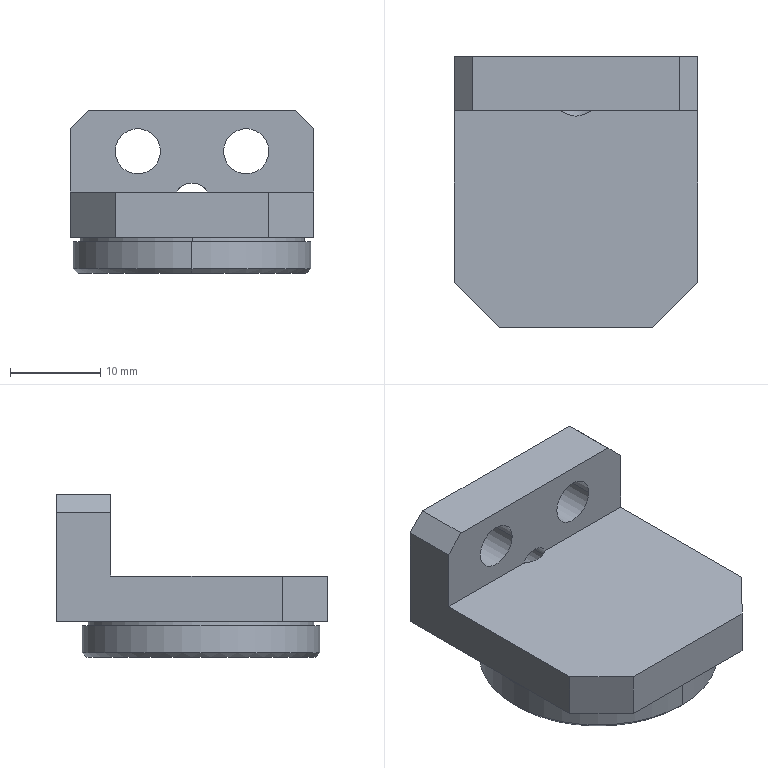NC program | NX | posted with a generic post | part box 27 x 30 x 18 mm
Whole program, first 1632 of 1946 lines:
N10 G17 G21 G94 G90
(FLOOR_WALL , TOOL : D10JING)
N12 T11 M6
N14 G54
N16 G17 G0 G90 X27. Y-17.497 B0. C0. S9500 M3
N18 G43 Z30. H11
N20 Z3.
N22 G94 G1 Z0. F1250.
N24 X24.
N26 X-24.
N28 Y-13.069
N30 X24.
N32 Y-8.641
N34 X-24.
N36 Y-4.213
N38 X24.
N40 Y0.216
N42 X-24.
N44 Y4.644
N46 X24.
N48 Y9.072
N50 X-24.
N52 Y13.5
N54 X24.
N56 X27.
N58 Z3.
N60 G0 Z30.
N62 M5
(ZLEVEL_PROFILE , TOOL : D10)
N64 T10 M6
N66 G54
N68 G17 G0 G90 X17.147 Y13.566 B0. C0. S9500 M3
N70 G43 Z30. H10
N72 Z1.5
N74 G94 G1 X18.832 Y11.88 Z1.375 F1000.
N76 X19.336 Y11.205 Z1.331
N78 X19.721 Y10.456 Z1.287
N80 X19.978 Y9.653 Z1.243
N82 X20.1 Y8.82 Z1.198
N84 Y-8.82 Z0.274
N86 X19.978 Y-9.653 Z0.23
N88 X19.721 Y-10.456 Z0.186
N90 X19.336 Y-11.205 Z0.142
N92 X18.832 Y-11.88 Z0.097
N94 X13.38 Y-17.332 Z-0.307
N96 X12.705 Y-17.836 Z-0.351
N98 X11.956 Y-18.221 Z-0.395
N100 X11.153 Y-18.478 Z-0.439
N102 X10.32 Y-18.6 Z-0.483
N104 X10. Z-0.5
N106 X-15. F3000.
N108 G2 X-20.1 Y-13.5 R5.1
N110 G1 Y13.5
N112 G2 X-15. Y18.6 R5.1
N114 G1 X10.
N116 G2 X13.606 Y17.106 R5.1
N118 G1 X18.606 Y12.106
N120 G2 X20.1 Y8.5 R5.1
N122 G1 Y-8.5
N124 G2 X18.606 Y-12.106 R5.1
N126 G1 X13.606 Y-17.106
N128 G2 X10. Y-18.6 R5.1
N130 G1 X-14.679 Z-0.931
N132 X-14.899 Z-0.935
N134 X-15.119 Y-18.599 Z-0.938
N136 X-15.34 Y-18.589 Z-0.942
N138 X-15.559 Y-18.569 Z-0.946
N140 X-15.777 Y-18.54 Z-0.95
N142 X-15.994 Y-18.502 Z-0.954
N144 X-16.21 Y-18.454 Z-0.958
N146 X-16.422 Y-18.398 Z-0.962
N148 X-16.633 Y-18.332 Z-0.965
N150 X-16.84 Y-18.257 Z-0.969
N152 X-17.044 Y-18.173 Z-0.973
N154 X-17.243 Y-18.08 Z-0.977
N156 X-17.439 Y-17.979 Z-0.981
N158 X-17.63 Y-17.869 Z-0.985
N160 X-17.817 Y-17.752 Z-0.988
N162 X-17.998 Y-17.626 Z-0.992
N164 X-18.173 Y-17.493 Z-0.996
N166 X-18.343 Y-17.352 Z-1.
N168 G2 X-20.1 Y-13.5 R5.1
N170 G1 Y13.5
N172 G2 X-15. Y18.6 R5.1
N174 G1 X10.
N176 G2 X13.606 Y17.106 R5.1
N178 G1 X18.606 Y12.106
N180 G2 X20.1 Y8.5 R5.1
N182 G1 Y-8.5
N184 G2 X18.606 Y-12.106 R5.1
N186 G1 X13.606 Y-17.106
N188 G2 X10. Y-18.6 R5.1
N190 G1 X-14.679 Z-1.431
N192 X-14.899 Z-1.435
N194 X-15.119 Y-18.599 Z-1.438
N196 X-15.34 Y-18.589 Z-1.442
N198 X-15.559 Y-18.569 Z-1.446
N200 X-15.777 Y-18.54 Z-1.45
N202 X-15.994 Y-18.502 Z-1.454
N204 X-16.21 Y-18.454 Z-1.458
N206 X-16.422 Y-18.398 Z-1.462
N208 X-16.633 Y-18.332 Z-1.465
N210 X-16.84 Y-18.257 Z-1.469
N212 X-17.044 Y-18.173 Z-1.473
N214 X-17.243 Y-18.08 Z-1.477
N216 X-17.439 Y-17.979 Z-1.481
N218 X-17.63 Y-17.869 Z-1.485
N220 X-17.817 Y-17.752 Z-1.488
N222 X-17.998 Y-17.626 Z-1.492
N224 X-18.173 Y-17.493 Z-1.496
N226 X-18.343 Y-17.352 Z-1.5
N228 G2 X-20.1 Y-13.5 R5.1
N230 G1 Y13.5
N232 G2 X-15. Y18.6 R5.1
N234 G1 X10.
N236 G2 X13.606 Y17.106 R5.1
N238 G1 X18.606 Y12.106
N240 G2 X20.1 Y8.5 R5.1
N242 G1 Y-8.5
N244 G2 X18.606 Y-12.106 R5.1
N246 G1 X13.606 Y-17.106
N248 G2 X10. Y-18.6 R5.1
N250 G1 X-14.679 Z-1.931
N252 X-14.899 Z-1.935
N254 X-15.119 Y-18.599 Z-1.938
N256 X-15.34 Y-18.589 Z-1.942
N258 X-15.559 Y-18.569 Z-1.946
N260 X-15.777 Y-18.54 Z-1.95
N262 X-15.994 Y-18.502 Z-1.954
N264 X-16.21 Y-18.454 Z-1.958
N266 X-16.422 Y-18.398 Z-1.962
N268 X-16.633 Y-18.332 Z-1.965
N270 X-16.84 Y-18.257 Z-1.969
N272 X-17.044 Y-18.173 Z-1.973
N274 X-17.243 Y-18.08 Z-1.977
N276 X-17.439 Y-17.979 Z-1.981
N278 X-17.63 Y-17.869 Z-1.985
N280 X-17.817 Y-17.752 Z-1.988
N282 X-17.998 Y-17.626 Z-1.992
N284 X-18.173 Y-17.493 Z-1.996
N286 X-18.343 Y-17.352 Z-2.
N288 G2 X-20.1 Y-13.5 R5.1
N290 G1 Y13.5
N292 G2 X-15. Y18.6 R5.1
N294 G1 X10.
N296 G2 X13.606 Y17.106 R5.1
N298 G1 X18.606 Y12.106
N300 G2 X20.1 Y8.5 R5.1
N302 G1 Y-8.5
N304 G2 X18.606 Y-12.106 R5.1
N306 G1 X13.606 Y-17.106
N308 G2 X10. Y-18.6 R5.1
N310 G1 X-14.679 Z-2.431
N312 X-14.899 Z-2.435
N314 X-15.119 Y-18.599 Z-2.438
N316 X-15.34 Y-18.589 Z-2.442
N318 X-15.559 Y-18.569 Z-2.446
N320 X-15.777 Y-18.54 Z-2.45
N322 X-15.994 Y-18.502 Z-2.454
N324 X-16.21 Y-18.454 Z-2.458
N326 X-16.422 Y-18.398 Z-2.462
N328 X-16.633 Y-18.332 Z-2.465
N330 X-16.84 Y-18.257 Z-2.469
N332 X-17.044 Y-18.173 Z-2.473
N334 X-17.243 Y-18.08 Z-2.477
N336 X-17.439 Y-17.979 Z-2.481
N338 X-17.63 Y-17.869 Z-2.485
N340 X-17.817 Y-17.752 Z-2.488
N342 X-17.998 Y-17.626 Z-2.492
N344 X-18.173 Y-17.493 Z-2.496
N346 X-18.343 Y-17.352 Z-2.5
N348 G2 X-20.1 Y-13.5 R5.1
N350 G1 Y13.5
N352 G2 X-15. Y18.6 R5.1
N354 G1 X10.
N356 G2 X13.606 Y17.106 R5.1
N358 G1 X18.606 Y12.106
N360 G2 X20.1 Y8.5 R5.1
N362 G1 Y-8.5
N364 G2 X18.606 Y-12.106 R5.1
N366 G1 X13.606 Y-17.106
N368 G2 X10. Y-18.6 R5.1
N370 G1 X-14.679 Z-2.931
N372 X-14.899 Z-2.935
N374 X-15.119 Y-18.599 Z-2.938
N376 X-15.34 Y-18.589 Z-2.942
N378 X-15.559 Y-18.569 Z-2.946
N380 X-15.777 Y-18.54 Z-2.95
N382 X-15.994 Y-18.502 Z-2.954
N384 X-16.21 Y-18.454 Z-2.958
N386 X-16.422 Y-18.398 Z-2.962
N388 X-16.633 Y-18.332 Z-2.965
N390 X-16.84 Y-18.257 Z-2.969
N392 X-17.044 Y-18.173 Z-2.973
N394 X-17.243 Y-18.08 Z-2.977
N396 X-17.439 Y-17.979 Z-2.981
N398 X-17.63 Y-17.869 Z-2.985
N400 X-17.817 Y-17.752 Z-2.988
N402 X-17.998 Y-17.626 Z-2.992
N404 X-18.173 Y-17.493 Z-2.996
N406 X-18.343 Y-17.352 Z-3.
N408 G2 X-20.1 Y-13.5 R5.1
N410 G1 Y13.5
N412 G2 X-15. Y18.6 R5.1
N414 G1 X10.
N416 G2 X13.606 Y17.106 R5.1
N418 G1 X18.606 Y12.106
N420 G2 X20.1 Y8.5 R5.1
N422 G1 Y-8.5
N424 G2 X18.606 Y-12.106 R5.1
N426 G1 X13.606 Y-17.106
N428 G2 X10. Y-18.6 R5.1
N430 G1 X-14.679 Z-3.431
N432 X-14.899 Z-3.435
N434 X-15.119 Y-18.599 Z-3.438
N436 X-15.34 Y-18.589 Z-3.442
N438 X-15.559 Y-18.569 Z-3.446
N440 X-15.777 Y-18.54 Z-3.45
N442 X-15.994 Y-18.502 Z-3.454
N444 X-16.21 Y-18.454 Z-3.458
N446 X-16.422 Y-18.398 Z-3.462
N448 X-16.633 Y-18.332 Z-3.465
N450 X-16.84 Y-18.257 Z-3.469
N452 X-17.044 Y-18.173 Z-3.473
N454 X-17.243 Y-18.08 Z-3.477
N456 X-17.439 Y-17.979 Z-3.481
N458 X-17.63 Y-17.869 Z-3.485
N460 X-17.817 Y-17.752 Z-3.488
N462 X-17.998 Y-17.626 Z-3.492
N464 X-18.173 Y-17.493 Z-3.496
N466 X-18.343 Y-17.352 Z-3.5
N468 G2 X-20.1 Y-13.5 R5.1
N470 G1 Y13.5
N472 G2 X-15. Y18.6 R5.1
N474 G1 X10.
N476 G2 X13.606 Y17.106 R5.1
N478 G1 X18.606 Y12.106
N480 G2 X20.1 Y8.5 R5.1
N482 G1 Y-8.5
N484 G2 X18.606 Y-12.106 R5.1
N486 G1 X13.606 Y-17.106
N488 G2 X10. Y-18.6 R5.1
N490 G1 X-14.679 Z-3.931
N492 X-14.899 Z-3.935
N494 X-15.119 Y-18.599 Z-3.938
N496 X-15.34 Y-18.589 Z-3.942
N498 X-15.559 Y-18.569 Z-3.946
N500 X-15.777 Y-18.54 Z-3.95
N502 X-15.994 Y-18.502 Z-3.954
N504 X-16.21 Y-18.454 Z-3.958
N506 X-16.422 Y-18.398 Z-3.962
N508 X-16.633 Y-18.332 Z-3.965
N510 X-16.84 Y-18.257 Z-3.969
N512 X-17.044 Y-18.173 Z-3.973
N514 X-17.243 Y-18.08 Z-3.977
N516 X-17.439 Y-17.979 Z-3.981
N518 X-17.63 Y-17.869 Z-3.985
N520 X-17.817 Y-17.752 Z-3.988
N522 X-17.998 Y-17.626 Z-3.992
N524 X-18.173 Y-17.493 Z-3.996
N526 X-18.343 Y-17.352 Z-4.
N528 G2 X-20.1 Y-13.5 R5.1
N530 G1 Y13.5
N532 G2 X-15. Y18.6 R5.1
N534 G1 X10.
N536 G2 X13.606 Y17.106 R5.1
N538 G1 X18.606 Y12.106
N540 G2 X20.1 Y8.5 R5.1
N542 G1 Y-8.5
N544 G2 X18.606 Y-12.106 R5.1
N546 G1 X13.606 Y-17.106
N548 G2 X10. Y-18.6 R5.1
N550 G1 X-14.679 Z-4.431
N552 X-14.899 Z-4.435
N554 X-15.119 Y-18.599 Z-4.438
N556 X-15.34 Y-18.589 Z-4.442
N558 X-15.559 Y-18.569 Z-4.446
N560 X-15.777 Y-18.54 Z-4.45
N562 X-15.994 Y-18.502 Z-4.454
N564 X-16.21 Y-18.454 Z-4.458
N566 X-16.422 Y-18.398 Z-4.462
N568 X-16.633 Y-18.332 Z-4.465
N570 X-16.84 Y-18.257 Z-4.469
N572 X-17.044 Y-18.173 Z-4.473
N574 X-17.243 Y-18.08 Z-4.477
N576 X-17.439 Y-17.979 Z-4.481
N578 X-17.63 Y-17.869 Z-4.485
N580 X-17.817 Y-17.752 Z-4.488
N582 X-17.998 Y-17.626 Z-4.492
N584 X-18.173 Y-17.493 Z-4.496
N586 X-18.343 Y-17.352 Z-4.5
N588 G2 X-20.1 Y-13.5 R5.1
N590 G1 Y13.5
N592 G2 X-15. Y18.6 R5.1
N594 G1 X10.
N596 G2 X13.606 Y17.106 R5.1
N598 G1 X18.606 Y12.106
N600 G2 X20.1 Y8.5 R5.1
N602 G1 Y-8.5
N604 G2 X18.606 Y-12.106 R5.1
N606 G1 X13.606 Y-17.106
N608 G2 X10. Y-18.6 R5.1
N610 G1 X-14.679 Z-4.931
N612 X-14.899 Z-4.935
N614 X-15.119 Y-18.599 Z-4.938
N616 X-15.34 Y-18.589 Z-4.942
N618 X-15.559 Y-18.569 Z-4.946
N620 X-15.777 Y-18.54 Z-4.95
N622 X-15.994 Y-18.502 Z-4.954
N624 X-16.21 Y-18.454 Z-4.958
N626 X-16.422 Y-18.398 Z-4.962
N628 X-16.633 Y-18.332 Z-4.965
N630 X-16.84 Y-18.257 Z-4.969
N632 X-17.044 Y-18.173 Z-4.973
N634 X-17.243 Y-18.08 Z-4.977
N636 X-17.439 Y-17.979 Z-4.981
N638 X-17.63 Y-17.869 Z-4.985
N640 X-17.817 Y-17.752 Z-4.988
N642 X-17.998 Y-17.626 Z-4.992
N644 X-18.173 Y-17.493 Z-4.996
N646 X-18.343 Y-17.352 Z-5.
N648 G2 X-20.1 Y-13.5 R5.1
N650 G1 Y13.5
N652 G2 X-15. Y18.6 R5.1
N654 G1 X10.
N656 G2 X13.606 Y17.106 R5.1
N658 G1 X18.606 Y12.106
N660 G2 X20.1 Y8.5 R5.1
N662 G1 Y-8.5
N664 G2 X18.606 Y-12.106 R5.1
N666 G1 X13.606 Y-17.106
N668 G2 X10. Y-18.6 R5.1
N670 G1 X-14.679 Z-5.431
N672 X-14.899 Z-5.435
N674 X-15.119 Y-18.599 Z-5.438
N676 X-15.34 Y-18.589 Z-5.442
N678 X-15.559 Y-18.569 Z-5.446
N680 X-15.777 Y-18.54 Z-5.45
N682 X-15.994 Y-18.502 Z-5.454
N684 X-16.21 Y-18.454 Z-5.458
N686 X-16.422 Y-18.398 Z-5.462
N688 X-16.633 Y-18.332 Z-5.465
N690 X-16.84 Y-18.257 Z-5.469
N692 X-17.044 Y-18.173 Z-5.473
N694 X-17.243 Y-18.08 Z-5.477
N696 X-17.439 Y-17.979 Z-5.481
N698 X-17.63 Y-17.869 Z-5.485
N700 X-17.817 Y-17.752 Z-5.488
N702 X-17.998 Y-17.626 Z-5.492
N704 X-18.173 Y-17.493 Z-5.496
N706 X-18.343 Y-17.352 Z-5.5
N708 G2 X-20.1 Y-13.5 R5.1
N710 G1 Y13.5
N712 G2 X-15. Y18.6 R5.1
N714 G1 X10.
N716 G2 X13.606 Y17.106 R5.1
N718 G1 X18.606 Y12.106
N720 G2 X20.1 Y8.5 R5.1
N722 G1 Y-8.5
N724 G2 X18.606 Y-12.106 R5.1
N726 G1 X13.606 Y-17.106
N728 G2 X10. Y-18.6 R5.1
N730 G1 X-14.679 Z-5.931
N732 X-14.899 Z-5.935
N734 X-15.119 Y-18.599 Z-5.938
N736 X-15.34 Y-18.589 Z-5.942
N738 X-15.559 Y-18.569 Z-5.946
N740 X-15.777 Y-18.54 Z-5.95
N742 X-15.994 Y-18.502 Z-5.954
N744 X-16.21 Y-18.454 Z-5.958
N746 X-16.422 Y-18.398 Z-5.962
N748 X-16.633 Y-18.332 Z-5.965
N750 X-16.84 Y-18.257 Z-5.969
N752 X-17.044 Y-18.173 Z-5.973
N754 X-17.243 Y-18.08 Z-5.977
N756 X-17.439 Y-17.979 Z-5.981
N758 X-17.63 Y-17.869 Z-5.985
N760 X-17.817 Y-17.752 Z-5.988
N762 X-17.998 Y-17.626 Z-5.992
N764 X-18.173 Y-17.493 Z-5.996
N766 X-18.343 Y-17.352 Z-6.
N768 G2 X-20.1 Y-13.5 R5.1
N770 G1 Y13.5
N772 G2 X-15. Y18.6 R5.1
N774 G1 X10.
N776 G2 X13.606 Y17.106 R5.1
N778 G1 X18.606 Y12.106
N780 G2 X20.1 Y8.5 R5.1
N782 G1 Y-8.5
N784 G2 X18.606 Y-12.106 R5.1
N786 G1 X13.606 Y-17.106
N788 G2 X10. Y-18.6 R5.1
N790 G1 X-14.679 Z-6.431
N792 X-14.899 Z-6.435
N794 X-15.119 Y-18.599 Z-6.438
N796 X-15.34 Y-18.589 Z-6.442
N798 X-15.559 Y-18.569 Z-6.446
N800 X-15.777 Y-18.54 Z-6.45
N802 X-15.994 Y-18.502 Z-6.454
N804 X-16.21 Y-18.454 Z-6.458
N806 X-16.422 Y-18.398 Z-6.462
N808 X-16.633 Y-18.332 Z-6.465
N810 X-16.84 Y-18.257 Z-6.469
N812 X-17.044 Y-18.173 Z-6.473
N814 X-17.243 Y-18.08 Z-6.477
N816 X-17.439 Y-17.979 Z-6.481
N818 X-17.63 Y-17.869 Z-6.485
N820 X-17.817 Y-17.752 Z-6.488
N822 X-17.998 Y-17.626 Z-6.492
N824 X-18.173 Y-17.493 Z-6.496
N826 X-18.343 Y-17.352 Z-6.5
N828 G2 X-20.1 Y-13.5 R5.1
N830 G1 Y13.5
N832 G2 X-15. Y18.6 R5.1
N834 G1 X10.
N836 G2 X13.606 Y17.106 R5.1
N838 G1 X18.606 Y12.106
N840 G2 X20.1 Y8.5 R5.1
N842 G1 Y-8.5
N844 G2 X18.606 Y-12.106 R5.1
N846 G1 X13.606 Y-17.106
N848 G2 X10. Y-18.6 R5.1
N850 G1 X-14.679 Z-6.931
N852 X-14.899 Z-6.935
N854 X-15.119 Y-18.599 Z-6.938
N856 X-15.34 Y-18.589 Z-6.942
N858 X-15.559 Y-18.569 Z-6.946
N860 X-15.777 Y-18.54 Z-6.95
N862 X-15.994 Y-18.502 Z-6.954
N864 X-16.21 Y-18.454 Z-6.958
N866 X-16.422 Y-18.398 Z-6.962
N868 X-16.633 Y-18.332 Z-6.965
N870 X-16.84 Y-18.257 Z-6.969
N872 X-17.044 Y-18.173 Z-6.973
N874 X-17.243 Y-18.08 Z-6.977
N876 X-17.439 Y-17.979 Z-6.981
N878 X-17.63 Y-17.869 Z-6.985
N880 X-17.817 Y-17.752 Z-6.988
N882 X-17.998 Y-17.626 Z-6.992
N884 X-18.173 Y-17.493 Z-6.996
N886 X-18.343 Y-17.352 Z-7.
N888 G2 X-20.1 Y-13.5 R5.1
N890 G1 Y13.5
N892 G2 X-15. Y18.6 R5.1
N894 G1 X10.
N896 G2 X13.606 Y17.106 R5.1
N898 G1 X18.606 Y12.106
N900 G2 X20.1 Y8.5 R5.1
N902 G1 Y-8.5
N904 G2 X18.606 Y-12.106 R5.1
N906 G1 X13.606 Y-17.106
N908 G2 X10. Y-18.6 R5.1
N910 G1 X-14.679 Z-7.431
N912 X-14.899 Z-7.435
N914 X-15.119 Y-18.599 Z-7.438
N916 X-15.34 Y-18.589 Z-7.442
N918 X-15.559 Y-18.569 Z-7.446
N920 X-15.777 Y-18.54 Z-7.45
N922 X-15.994 Y-18.502 Z-7.454
N924 X-16.21 Y-18.454 Z-7.458
N926 X-16.422 Y-18.398 Z-7.462
N928 X-16.633 Y-18.332 Z-7.465
N930 X-16.84 Y-18.257 Z-7.469
N932 X-17.044 Y-18.173 Z-7.473
N934 X-17.243 Y-18.08 Z-7.477
N936 X-17.439 Y-17.979 Z-7.481
N938 X-17.63 Y-17.869 Z-7.485
N940 X-17.817 Y-17.752 Z-7.488
N942 X-17.998 Y-17.626 Z-7.492
N944 X-18.173 Y-17.493 Z-7.496
N946 X-18.343 Y-17.352 Z-7.5
N948 G2 X-20.1 Y-13.5 R5.1
N950 G1 Y13.5
N952 G2 X-15. Y18.6 R5.1
N954 G1 X10.
N956 G2 X13.606 Y17.106 R5.1
N958 G1 X18.606 Y12.106
N960 G2 X20.1 Y8.5 R5.1
N962 G1 Y-8.5
N964 G2 X18.606 Y-12.106 R5.1
N966 G1 X13.606 Y-17.106
N968 G2 X10. Y-18.6 R5.1
N970 G1 X-14.679 Z-7.931
N972 X-14.899 Z-7.935
N974 X-15.119 Y-18.599 Z-7.938
N976 X-15.34 Y-18.589 Z-7.942
N978 X-15.559 Y-18.569 Z-7.946
N980 X-15.777 Y-18.54 Z-7.95
N982 X-15.994 Y-18.502 Z-7.954
N984 X-16.21 Y-18.454 Z-7.958
N986 X-16.422 Y-18.398 Z-7.962
N988 X-16.633 Y-18.332 Z-7.965
N990 X-16.84 Y-18.257 Z-7.969
N992 X-17.044 Y-18.173 Z-7.973
N994 X-17.243 Y-18.08 Z-7.977
N996 X-17.439 Y-17.979 Z-7.981
N998 X-17.63 Y-17.869 Z-7.985
N1000 X-17.817 Y-17.752 Z-7.988
N1002 X-17.998 Y-17.626 Z-7.992
N1004 X-18.173 Y-17.493 Z-7.996
N1006 X-18.343 Y-17.352 Z-8.
N1008 G2 X-20.1 Y-13.5 R5.1
N1010 G1 Y13.5
N1012 G2 X-15. Y18.6 R5.1
N1014 G1 X10.
N1016 G2 X13.606 Y17.106 R5.1
N1018 G1 X18.606 Y12.106
N1020 G2 X20.1 Y8.5 R5.1
N1022 G1 Y-8.5
N1024 G2 X18.606 Y-12.106 R5.1
N1026 G1 X13.606 Y-17.106
N1028 G2 X10. Y-18.6 R5.1
N1030 G1 X-14.679 Z-8.431
N1032 X-14.899 Z-8.435
N1034 X-15.119 Y-18.599 Z-8.438
N1036 X-15.34 Y-18.589 Z-8.442
N1038 X-15.559 Y-18.569 Z-8.446
N1040 X-15.777 Y-18.54 Z-8.45
N1042 X-15.994 Y-18.502 Z-8.454
N1044 X-16.21 Y-18.454 Z-8.458
N1046 X-16.422 Y-18.398 Z-8.462
N1048 X-16.633 Y-18.332 Z-8.465
N1050 X-16.84 Y-18.257 Z-8.469
N1052 X-17.044 Y-18.173 Z-8.473
N1054 X-17.243 Y-18.08 Z-8.477
N1056 X-17.439 Y-17.979 Z-8.481
N1058 X-17.63 Y-17.869 Z-8.485
N1060 X-17.817 Y-17.752 Z-8.488
N1062 X-17.998 Y-17.626 Z-8.492
N1064 X-18.173 Y-17.493 Z-8.496
N1066 X-18.343 Y-17.352 Z-8.5
N1068 G2 X-20.1 Y-13.5 R5.1
N1070 G1 Y13.5
N1072 G2 X-15. Y18.6 R5.1
N1074 G1 X10.
N1076 G2 X13.606 Y17.106 R5.1
N1078 G1 X18.606 Y12.106
N1080 G2 X20.1 Y8.5 R5.1
N1082 G1 Y-8.5
N1084 G2 X18.606 Y-12.106 R5.1
N1086 G1 X13.606 Y-17.106
N1088 G2 X10. Y-18.6 R5.1
N1090 G1 X-14.679 Z-8.931
N1092 X-14.899 Z-8.935
N1094 X-15.119 Y-18.599 Z-8.938
N1096 X-15.34 Y-18.589 Z-8.942
N1098 X-15.559 Y-18.569 Z-8.946
N1100 X-15.777 Y-18.54 Z-8.95
N1102 X-15.994 Y-18.502 Z-8.954
N1104 X-16.21 Y-18.454 Z-8.958
N1106 X-16.422 Y-18.398 Z-8.962
N1108 X-16.633 Y-18.332 Z-8.965
N1110 X-16.84 Y-18.257 Z-8.969
N1112 X-17.044 Y-18.173 Z-8.973
N1114 X-17.243 Y-18.08 Z-8.977
N1116 X-17.439 Y-17.979 Z-8.981
N1118 X-17.63 Y-17.869 Z-8.985
N1120 X-17.817 Y-17.752 Z-8.988
N1122 X-17.998 Y-17.626 Z-8.992
N1124 X-18.173 Y-17.493 Z-8.996
N1126 X-18.343 Y-17.352 Z-9.
N1128 G2 X-20.1 Y-13.5 R5.1
N1130 G1 Y13.5
N1132 G2 X-15. Y18.6 R5.1
N1134 G1 X10.
N1136 G2 X13.606 Y17.106 R5.1
N1138 G1 X18.606 Y12.106
N1140 G2 X20.1 Y8.5 R5.1
N1142 G1 Y-8.5
N1144 G2 X18.606 Y-12.106 R5.1
N1146 G1 X13.606 Y-17.106
N1148 G2 X10. Y-18.6 R5.1
N1150 G1 X-14.679 Z-9.431
N1152 X-14.899 Z-9.435
N1154 X-15.119 Y-18.599 Z-9.438
N1156 X-15.34 Y-18.589 Z-9.442
N1158 X-15.559 Y-18.569 Z-9.446
N1160 X-15.777 Y-18.54 Z-9.45
N1162 X-15.994 Y-18.502 Z-9.454
N1164 X-16.21 Y-18.454 Z-9.458
N1166 X-16.422 Y-18.398 Z-9.462
N1168 X-16.633 Y-18.332 Z-9.465
N1170 X-16.84 Y-18.257 Z-9.469
N1172 X-17.044 Y-18.173 Z-9.473
N1174 X-17.243 Y-18.08 Z-9.477
N1176 X-17.439 Y-17.979 Z-9.481
N1178 X-17.63 Y-17.869 Z-9.485
N1180 X-17.817 Y-17.752 Z-9.488
N1182 X-17.998 Y-17.626 Z-9.492
N1184 X-18.173 Y-17.493 Z-9.496
N1186 X-18.343 Y-17.352 Z-9.5
N1188 G2 X-20.1 Y-13.5 R5.1
N1190 G1 Y13.5
N1192 G2 X-15. Y18.6 R5.1
N1194 G1 X10.
N1196 G2 X13.606 Y17.106 R5.1
N1198 G1 X18.606 Y12.106
N1200 G2 X20.1 Y8.5 R5.1
N1202 G1 Y-8.5
N1204 G2 X18.606 Y-12.106 R5.1
N1206 G1 X13.606 Y-17.106
N1208 G2 X10. Y-18.6 R5.1
N1210 G1 X-14.679 Z-9.931
N1212 X-14.899 Z-9.935
N1214 X-15.119 Y-18.599 Z-9.938
N1216 X-15.34 Y-18.589 Z-9.942
N1218 X-15.559 Y-18.569 Z-9.946
N1220 X-15.777 Y-18.54 Z-9.95
N1222 X-15.994 Y-18.502 Z-9.954
N1224 X-16.21 Y-18.454 Z-9.958
N1226 X-16.422 Y-18.398 Z-9.962
N1228 X-16.633 Y-18.332 Z-9.965
N1230 X-16.84 Y-18.257 Z-9.969
N1232 X-17.044 Y-18.173 Z-9.973
N1234 X-17.243 Y-18.08 Z-9.977
N1236 X-17.439 Y-17.979 Z-9.981
N1238 X-17.63 Y-17.869 Z-9.985
N1240 X-17.817 Y-17.752 Z-9.988
N1242 X-17.998 Y-17.626 Z-9.992
N1244 X-18.173 Y-17.493 Z-9.996
N1246 X-18.343 Y-17.352 Z-10.
N1248 G2 X-20.1 Y-13.5 R5.1
N1250 G1 Y13.5
N1252 G2 X-15. Y18.6 R5.1
N1254 G1 X10.
N1256 G2 X13.606 Y17.106 R5.1
N1258 G1 X18.606 Y12.106
N1260 G2 X20.1 Y8.5 R5.1
N1262 G1 Y-8.5
N1264 G2 X18.606 Y-12.106 R5.1
N1266 G1 X13.606 Y-17.106
N1268 G2 X10. Y-18.6 R5.1
N1270 G1 X-14.679 Z-10.431
N1272 X-14.899 Z-10.435
N1274 X-15.119 Y-18.599 Z-10.438
N1276 X-15.34 Y-18.589 Z-10.442
N1278 X-15.559 Y-18.569 Z-10.446
N1280 X-15.777 Y-18.54 Z-10.45
N1282 X-15.994 Y-18.502 Z-10.454
N1284 X-16.21 Y-18.454 Z-10.458
N1286 X-16.422 Y-18.398 Z-10.462
N1288 X-16.633 Y-18.332 Z-10.465
N1290 X-16.84 Y-18.257 Z-10.469
N1292 X-17.044 Y-18.173 Z-10.473
N1294 X-17.243 Y-18.08 Z-10.477
N1296 X-17.439 Y-17.979 Z-10.481
N1298 X-17.63 Y-17.869 Z-10.485
N1300 X-17.817 Y-17.752 Z-10.488
N1302 X-17.998 Y-17.626 Z-10.492
N1304 X-18.173 Y-17.493 Z-10.496
N1306 X-18.343 Y-17.352 Z-10.5
N1308 G2 X-20.1 Y-13.5 R5.1
N1310 G1 Y13.5
N1312 G2 X-15. Y18.6 R5.1
N1314 G1 X10.
N1316 G2 X13.606 Y17.106 R5.1
N1318 G1 X18.606 Y12.106
N1320 G2 X20.1 Y8.5 R5.1
N1322 G1 Y-8.5
N1324 G2 X18.606 Y-12.106 R5.1
N1326 G1 X13.606 Y-17.106
N1328 G2 X10. Y-18.6 R5.1
N1330 G1 X-14.679 Z-10.931
N1332 X-14.899 Z-10.935
N1334 X-15.119 Y-18.599 Z-10.938
N1336 X-15.34 Y-18.589 Z-10.942
N1338 X-15.559 Y-18.569 Z-10.946
N1340 X-15.777 Y-18.54 Z-10.95
N1342 X-15.994 Y-18.502 Z-10.954
N1344 X-16.21 Y-18.454 Z-10.958
N1346 X-16.422 Y-18.398 Z-10.962
N1348 X-16.633 Y-18.332 Z-10.965
N1350 X-16.84 Y-18.257 Z-10.969
N1352 X-17.044 Y-18.173 Z-10.973
N1354 X-17.243 Y-18.08 Z-10.977
N1356 X-17.439 Y-17.979 Z-10.981
N1358 X-17.63 Y-17.869 Z-10.985
N1360 X-17.817 Y-17.752 Z-10.988
N1362 X-17.998 Y-17.626 Z-10.992
N1364 X-18.173 Y-17.493 Z-10.996
N1366 X-18.343 Y-17.352 Z-11.
N1368 G2 X-20.1 Y-13.5 R5.1
N1370 G1 Y13.5
N1372 G2 X-15. Y18.6 R5.1
N1374 G1 X10.
N1376 G2 X13.606 Y17.106 R5.1
N1378 G1 X18.606 Y12.106
N1380 G2 X20.1 Y8.5 R5.1
N1382 G1 Y-8.5
N1384 G2 X18.606 Y-12.106 R5.1
N1386 G1 X13.606 Y-17.106
N1388 G2 X10. Y-18.6 R5.1
N1390 G1 X-14.679 Z-11.431
N1392 X-14.899 Z-11.435
N1394 X-15.119 Y-18.599 Z-11.438
N1396 X-15.34 Y-18.589 Z-11.442
N1398 X-15.559 Y-18.569 Z-11.446
N1400 X-15.777 Y-18.54 Z-11.45
N1402 X-15.994 Y-18.502 Z-11.454
N1404 X-16.21 Y-18.454 Z-11.458
N1406 X-16.422 Y-18.398 Z-11.462
N1408 X-16.633 Y-18.332 Z-11.465
N1410 X-16.84 Y-18.257 Z-11.469
N1412 X-17.044 Y-18.173 Z-11.473
N1414 X-17.243 Y-18.08 Z-11.477
N1416 X-17.439 Y-17.979 Z-11.481
N1418 X-17.63 Y-17.869 Z-11.485
N1420 X-17.817 Y-17.752 Z-11.488
N1422 X-17.998 Y-17.626 Z-11.492
N1424 X-18.173 Y-17.493 Z-11.496
N1426 X-18.343 Y-17.352 Z-11.5
N1428 G2 X-20.1 Y-13.5 R5.1
N1430 G1 Y13.5
N1432 G2 X-15. Y18.6 R5.1
N1434 G1 X10.
N1436 G2 X13.606 Y17.106 R5.1
N1438 G1 X18.606 Y12.106
N1440 G2 X20.1 Y8.5 R5.1
N1442 G1 Y-8.5
N1444 G2 X18.606 Y-12.106 R5.1
N1446 G1 X13.606 Y-17.106
N1448 G2 X10. Y-18.6 R5.1
N1450 G1 X-14.679 Z-11.931
N1452 X-14.899 Z-11.935
N1454 X-15.119 Y-18.599 Z-11.938
N1456 X-15.34 Y-18.589 Z-11.942
N1458 X-15.559 Y-18.569 Z-11.946
N1460 X-15.777 Y-18.54 Z-11.95
N1462 X-15.994 Y-18.502 Z-11.954
N1464 X-16.21 Y-18.454 Z-11.958
N1466 X-16.422 Y-18.398 Z-11.962
N1468 X-16.633 Y-18.332 Z-11.965
N1470 X-16.84 Y-18.257 Z-11.969
N1472 X-17.044 Y-18.173 Z-11.973
N1474 X-17.243 Y-18.08 Z-11.977
N1476 X-17.439 Y-17.979 Z-11.981
N1478 X-17.63 Y-17.869 Z-11.985
N1480 X-17.817 Y-17.752 Z-11.988
N1482 X-17.998 Y-17.626 Z-11.992
N1484 X-18.173 Y-17.493 Z-11.996
N1486 X-18.343 Y-17.352 Z-12.
N1488 G2 X-20.1 Y-13.5 R5.1
N1490 G1 Y13.5
N1492 G2 X-15. Y18.6 R5.1
N1494 G1 X10.
N1496 G2 X13.606 Y17.106 R5.1
N1498 G1 X18.606 Y12.106
N1500 G2 X20.1 Y8.5 R5.1
N1502 G1 Y-8.5
N1504 G2 X18.606 Y-12.106 R5.1
N1506 G1 X13.606 Y-17.106
N1508 G2 X10. Y-18.6 R5.1
N1510 G1 X-14.679 Z-12.431
N1512 X-14.899 Z-12.435
N1514 X-15.119 Y-18.599 Z-12.438
N1516 X-15.34 Y-18.589 Z-12.442
N1518 X-15.559 Y-18.569 Z-12.446
N1520 X-15.777 Y-18.54 Z-12.45
N1522 X-15.994 Y-18.502 Z-12.454
N1524 X-16.21 Y-18.454 Z-12.458
N1526 X-16.422 Y-18.398 Z-12.462
N1528 X-16.633 Y-18.332 Z-12.465
N1530 X-16.84 Y-18.257 Z-12.469
N1532 X-17.044 Y-18.173 Z-12.473
N1534 X-17.243 Y-18.08 Z-12.477
N1536 X-17.439 Y-17.979 Z-12.481
N1538 X-17.63 Y-17.869 Z-12.485
N1540 X-17.817 Y-17.752 Z-12.488
N1542 X-17.998 Y-17.626 Z-12.492
N1544 X-18.173 Y-17.493 Z-12.496
N1546 X-18.343 Y-17.352 Z-12.5
N1548 G2 X-20.1 Y-13.5 R5.1
N1550 G1 Y13.5
N1552 G2 X-15. Y18.6 R5.1
N1554 G1 X10.
N1556 G2 X13.606 Y17.106 R5.1
N1558 G1 X18.606 Y12.106
N1560 G2 X20.1 Y8.5 R5.1
N1562 G1 Y-8.5
N1564 G2 X18.606 Y-12.106 R5.1
N1566 G1 X13.606 Y-17.106
N1568 G2 X10. Y-18.6 R5.1
N1570 G1 X-14.679 Z-12.931
N1572 X-14.899 Z-12.935
N1574 X-15.119 Y-18.599 Z-12.938
N1576 X-15.34 Y-18.589 Z-12.942
N1578 X-15.559 Y-18.569 Z-12.946
N1580 X-15.777 Y-18.54 Z-12.95
N1582 X-15.994 Y-18.502 Z-12.954
N1584 X-16.21 Y-18.454 Z-12.958
N1586 X-16.422 Y-18.398 Z-12.962
N1588 X-16.633 Y-18.332 Z-12.965
N1590 X-16.84 Y-18.257 Z-12.969
N1592 X-17.044 Y-18.173 Z-12.973
N1594 X-17.243 Y-18.08 Z-12.977
N1596 X-17.439 Y-17.979 Z-12.981
N1598 X-17.63 Y-17.869 Z-12.985
N1600 X-17.817 Y-17.752 Z-12.988
N1602 X-17.998 Y-17.626 Z-12.992
N1604 X-18.173 Y-17.493 Z-12.996
N1606 X-18.343 Y-17.352 Z-13.
N1608 G2 X-20.1 Y-13.5 R5.1
N1610 G1 Y13.5
N1612 G2 X-15. Y18.6 R5.1
N1614 G1 X10.
N1616 G2 X13.606 Y17.106 R5.1
N1618 G1 X18.606 Y12.106
N1620 G2 X20.1 Y8.5 R5.1
N1622 G1 Y-8.5
N1624 G2 X18.606 Y-12.106 R5.1
N1626 G1 X13.606 Y-17.106
N1628 G2 X10. Y-18.6 R5.1
N1630 G1 X-14.679 Z-13.431
N1632 X-14.899 Z-13.435
N1634 X-15.119 Y-18.599 Z-13.438
N1636 X-15.34 Y-18.589 Z-13.442
N1638 X-15.559 Y-18.569 Z-13.446
N1640 X-15.777 Y-18.54 Z-13.45
N1642 X-15.994 Y-18.502 Z-13.454
N1644 X-16.21 Y-18.454 Z-13.458
N1646 X-16.422 Y-18.398 Z-13.462
N1648 X-16.633 Y-18.332 Z-13.465
N1650 X-16.84 Y-18.257 Z-13.469
N1652 X-17.044 Y-18.173 Z-13.473
N1654 X-17.243 Y-18.08 Z-13.477
N1656 X-17.439 Y-17.979 Z-13.481
N1658 X-17.63 Y-17.869 Z-13.485
N1660 X-17.817 Y-17.752 Z-13.488
N1662 X-17.998 Y-17.626 Z-13.492
N1664 X-18.173 Y-17.493 Z-13.496
N1666 X-18.343 Y-17.352 Z-13.5
N1668 G2 X-20.1 Y-13.5 R5.1
N1670 G1 Y13.5
N1672 G2 X-15. Y18.6 R5.1
N1674 G1 X10.
N1676 G2 X13.606 Y17.106 R5.1
N1678 G1 X18.606 Y12.106
N1680 G2 X20.1 Y8.5 R5.1
N1682 G1 Y-8.5
N1684 G2 X18.606 Y-12.106 R5.1
N1686 G1 X13.606 Y-17.106
N1688 G2 X10. Y-18.6 R5.1
N1690 G1 X-14.679 Z-13.931
N1692 X-14.899 Z-13.935
N1694 X-15.119 Y-18.599 Z-13.938
N1696 X-15.34 Y-18.589 Z-13.942
N1698 X-15.559 Y-18.569 Z-13.946
N1700 X-15.777 Y-18.54 Z-13.95
N1702 X-15.994 Y-18.502 Z-13.954
N1704 X-16.21 Y-18.454 Z-13.958
N1706 X-16.422 Y-18.398 Z-13.962
N1708 X-16.633 Y-18.332 Z-13.965
N1710 X-16.84 Y-18.257 Z-13.969
N1712 X-17.044 Y-18.173 Z-13.973
N1714 X-17.243 Y-18.08 Z-13.977
N1716 X-17.439 Y-17.979 Z-13.981
N1718 X-17.63 Y-17.869 Z-13.985
N1720 X-17.817 Y-17.752 Z-13.988
N1722 X-17.998 Y-17.626 Z-13.992
N1724 X-18.173 Y-17.493 Z-13.996
N1726 X-18.343 Y-17.352 Z-14.
N1728 G2 X-20.1 Y-13.5 R5.1
N1730 G1 Y13.5
N1732 G2 X-15. Y18.6 R5.1
N1734 G1 X10.
N1736 G2 X13.606 Y17.106 R5.1
N1738 G1 X18.606 Y12.106
N1740 G2 X20.1 Y8.5 R5.1
N1742 G1 Y-8.5
N1744 G2 X18.606 Y-12.106 R5.1
N1746 G1 X13.606 Y-17.106
N1748 G2 X10. Y-18.6 R5.1
N1750 G1 X-14.679 Z-14.431
N1752 X-14.899 Z-14.435
N1754 X-15.119 Y-18.599 Z-14.438
N1756 X-15.34 Y-18.589 Z-14.442
N1758 X-15.559 Y-18.569 Z-14.446
N1760 X-15.777 Y-18.54 Z-14.45
N1762 X-15.994 Y-18.502 Z-14.454
N1764 X-16.21 Y-18.454 Z-14.458
N1766 X-16.422 Y-18.398 Z-14.462
N1768 X-16.633 Y-18.332 Z-14.465
N1770 X-16.84 Y-18.257 Z-14.469
N1772 X-17.044 Y-18.173 Z-14.473
N1774 X-17.243 Y-18.08 Z-14.477
N1776 X-17.439 Y-17.979 Z-14.481
N1778 X-17.63 Y-17.869 Z-14.485
N1780 X-17.817 Y-17.752 Z-14.488
N1782 X-17.998 Y-17.626 Z-14.492
N1784 X-18.173 Y-17.493 Z-14.496
N1786 X-18.343 Y-17.352 Z-14.5
N1788 G2 X-20.1 Y-13.5 R5.1
N1790 G1 Y13.5
N1792 G2 X-15. Y18.6 R5.1
N1794 G1 X10.
N1796 G2 X13.606 Y17.106 R5.1
N1798 G1 X18.606 Y12.106
N1800 G2 X20.1 Y8.5 R5.1
N1802 G1 Y-8.5
N1804 G2 X18.606 Y-12.106 R5.1
N1806 G1 X13.606 Y-17.106
N1808 G2 X10. Y-18.6 R5.1
N1810 G1 X-14.679 Z-14.931
N1812 X-14.899 Z-14.935
N1814 X-15.119 Y-18.599 Z-14.938
N1816 X-15.34 Y-18.589 Z-14.942
N1818 X-15.559 Y-18.569 Z-14.946
N1820 X-15.777 Y-18.54 Z-14.95
N1822 X-15.994 Y-18.502 Z-14.954
N1824 X-16.21 Y-18.454 Z-14.958
N1826 X-16.422 Y-18.398 Z-14.962
N1828 X-16.633 Y-18.332 Z-14.965
N1830 X-16.84 Y-18.257 Z-14.969
N1832 X-17.044 Y-18.173 Z-14.973
N1834 X-17.243 Y-18.08 Z-14.977
N1836 X-17.439 Y-17.979 Z-14.981
N1838 X-17.63 Y-17.869 Z-14.985
N1840 X-17.817 Y-17.752 Z-14.988
N1842 X-17.998 Y-17.626 Z-14.992
N1844 X-18.173 Y-17.493 Z-14.996
N1846 X-18.343 Y-17.352 Z-15.
N1848 G2 X-20.1 Y-13.5 R5.1
N1850 G1 Y13.5
N1852 G2 X-15. Y18.6 R5.1
N1854 G1 X10.
N1856 G2 X13.606 Y17.106 R5.1
N1858 G1 X18.606 Y12.106
N1860 G2 X20.1 Y8.5 R5.1
N1862 G1 Y-8.5
N1864 G2 X18.606 Y-12.106 R5.1
N1866 G1 X13.606 Y-17.106
N1868 G2 X10. Y-18.6 R5.1
N1870 G1 X-14.679 Z-15.431
N1872 X-14.899 Z-15.435
N1874 X-15.119 Y-18.599 Z-15.438
N1876 X-15.34 Y-18.589 Z-15.442
N1878 X-15.559 Y-18.569 Z-15.446
N1880 X-15.777 Y-18.54 Z-15.45
N1882 X-15.994 Y-18.502 Z-15.454
N1884 X-16.21 Y-18.454 Z-15.458
N1886 X-16.422 Y-18.398 Z-15.462
N1888 X-16.633 Y-18.332 Z-15.465
N1890 X-16.84 Y-18.257 Z-15.469
N1892 X-17.044 Y-18.173 Z-15.473
N1894 X-17.243 Y-18.08 Z-15.477
N1896 X-17.439 Y-17.979 Z-15.481
N1898 X-17.63 Y-17.869 Z-15.485
N1900 X-17.817 Y-17.752 Z-15.488
N1902 X-17.998 Y-17.626 Z-15.492
N1904 X-18.173 Y-17.493 Z-15.496
N1906 X-18.343 Y-17.352 Z-15.5
N1908 G2 X-20.1 Y-13.5 R5.1
N1910 G1 Y13.5
N1912 G2 X-15. Y18.6 R5.1
N1914 G1 X10.
N1916 G2 X13.606 Y17.106 R5.1
N1918 G1 X18.606 Y12.106
N1920 G2 X20.1 Y8.5 R5.1
N1922 G1 Y-8.5
N1924 G2 X18.606 Y-12.106 R5.1
N1926 G1 X13.606 Y-17.106
N1928 G2 X10. Y-18.6 R5.1
N1930 G1 X-14.679 Z-15.931
N1932 X-14.899 Z-15.935
N1934 X-15.119 Y-18.599 Z-15.938
N1936 X-15.34 Y-18.589 Z-15.942
N1938 X-15.559 Y-18.569 Z-15.946
N1940 X-15.777 Y-18.54 Z-15.95
N1942 X-15.994 Y-18.502 Z-15.954
N1944 X-16.21 Y-18.454 Z-15.958
N1946 X-16.422 Y-18.398 Z-15.962
N1948 X-16.633 Y-18.332 Z-15.965
N1950 X-16.84 Y-18.257 Z-15.969
N1952 X-17.044 Y-18.173 Z-15.973
N1954 X-17.243 Y-18.08 Z-15.977
N1956 X-17.439 Y-17.979 Z-15.981
N1958 X-17.63 Y-17.869 Z-15.985
N1960 X-17.817 Y-17.752 Z-15.988
N1962 X-17.998 Y-17.626 Z-15.992
N1964 X-18.173 Y-17.493 Z-15.996
N1966 X-18.343 Y-17.352 Z-16.
N1968 G2 X-20.1 Y-13.5 R5.1
N1970 G1 Y13.5
N1972 G2 X-15. Y18.6 R5.1
N1974 G1 X10.
N1976 G2 X13.606 Y17.106 R5.1
N1978 G1 X18.606 Y12.106
N1980 G2 X20.1 Y8.5 R5.1
N1982 G1 Y-8.5
N1984 G2 X18.606 Y-12.106 R5.1
N1986 G1 X13.606 Y-17.106
N1988 G2 X10. Y-18.6 R5.1
N1990 G1 X-14.679 Z-16.431
N1992 X-14.899 Z-16.435
N1994 X-15.119 Y-18.599 Z-16.438
N1996 X-15.34 Y-18.589 Z-16.442
N1998 X-15.559 Y-18.569 Z-16.446
N2000 X-15.777 Y-18.54 Z-16.45
N2002 X-15.994 Y-18.502 Z-16.454
N2004 X-16.21 Y-18.454 Z-16.458
N2006 X-16.422 Y-18.398 Z-16.462
N2008 X-16.633 Y-18.332 Z-16.465
N2010 X-16.84 Y-18.257 Z-16.469
N2012 X-17.044 Y-18.173 Z-16.473
N2014 X-17.243 Y-18.08 Z-16.477
N2016 X-17.439 Y-17.979 Z-16.481
N2018 X-17.63 Y-17.869 Z-16.485
N2020 X-17.817 Y-17.752 Z-16.488
N2022 X-17.998 Y-17.626 Z-16.492
N2024 X-18.173 Y-17.493 Z-16.496
N2026 X-18.343 Y-17.352 Z-16.5
N2028 G2 X-20.1 Y-13.5 R5.1
N2030 G1 Y13.5
N2032 G2 X-15. Y18.6 R5.1
N2034 G1 X10.
N2036 G2 X13.606 Y17.106 R5.1
N2038 G1 X18.606 Y12.106
N2040 G2 X20.1 Y8.5 R5.1
N2042 G1 Y-8.5
N2044 G2 X18.606 Y-12.106 R5.1
N2046 G1 X13.606 Y-17.106
N2048 G2 X10. Y-18.6 R5.1
N2050 G1 X-14.679 Z-16.931
N2052 X-14.899 Z-16.935
N2054 X-15.119 Y-18.599 Z-16.938
N2056 X-15.34 Y-18.589 Z-16.942
N2058 X-15.559 Y-18.569 Z-16.946
N2060 X-15.777 Y-18.54 Z-16.95
N2062 X-15.994 Y-18.502 Z-16.954
N2064 X-16.21 Y-18.454 Z-16.958
N2066 X-16.422 Y-18.398 Z-16.962
N2068 X-16.633 Y-18.332 Z-16.965
N2070 X-16.84 Y-18.257 Z-16.969
N2072 X-17.044 Y-18.173 Z-16.973
N2074 X-17.243 Y-18.08 Z-16.977
N2076 X-17.439 Y-17.979 Z-16.981
N2078 X-17.63 Y-17.869 Z-16.985
N2080 X-17.817 Y-17.752 Z-16.988
N2082 X-17.998 Y-17.626 Z-16.992
N2084 X-18.173 Y-17.493 Z-16.996
N2086 X-18.343 Y-17.352 Z-17.
N2088 G2 X-20.1 Y-13.5 R5.1
N2090 G1 Y13.5
N2092 G2 X-15. Y18.6 R5.1
N2094 G1 X10.
N2096 G2 X13.606 Y17.106 R5.1
N2098 G1 X18.606 Y12.106
N2100 G2 X20.1 Y8.5 R5.1
N2102 G1 Y-8.5
N2104 G2 X18.606 Y-12.106 R5.1
N2106 G1 X13.606 Y-17.106
N2108 G2 X10. Y-18.6 R5.1
N2110 G1 X-14.679 Z-17.431
N2112 X-14.899 Z-17.435
N2114 X-15.119 Y-18.599 Z-17.438
N2116 X-15.34 Y-18.589 Z-17.442
N2118 X-15.559 Y-18.569 Z-17.446
N2120 X-15.777 Y-18.54 Z-17.45
N2122 X-15.994 Y-18.502 Z-17.454
N2124 X-16.21 Y-18.454 Z-17.458
N2126 X-16.422 Y-18.398 Z-17.462
N2128 X-16.633 Y-18.332 Z-17.465
N2130 X-16.84 Y-18.257 Z-17.469
N2132 X-17.044 Y-18.173 Z-17.473
N2134 X-17.243 Y-18.08 Z-17.477
N2136 X-17.439 Y-17.979 Z-17.481
N2138 X-17.63 Y-17.869 Z-17.485
N2140 X-17.817 Y-17.752 Z-17.488
N2142 X-17.998 Y-17.626 Z-17.492
N2144 X-18.173 Y-17.493 Z-17.496
N2146 X-18.343 Y-17.352 Z-17.5
N2148 G2 X-20.1 Y-13.5 R5.1
N2150 G1 Y13.5
N2152 G2 X-15. Y18.6 R5.1
N2154 G1 X10.
N2156 G2 X13.606 Y17.106 R5.1
N2158 G1 X18.606 Y12.106
N2160 G2 X20.1 Y8.5 R5.1
N2162 G1 Y-8.5
N2164 G2 X18.606 Y-12.106 R5.1
N2166 G1 X13.606 Y-17.106
N2168 G2 X10. Y-18.6 R5.1
N2170 G1 X-14.679 Z-17.931
N2172 X-14.899 Z-17.935
N2174 X-15.119 Y-18.599 Z-17.938
N2176 X-15.34 Y-18.589 Z-17.942
N2178 X-15.559 Y-18.569 Z-17.946
N2180 X-15.777 Y-18.54 Z-17.95
N2182 X-15.994 Y-18.502 Z-17.954
N2184 X-16.21 Y-18.454 Z-17.958
N2186 X-16.422 Y-18.398 Z-17.962
N2188 X-16.633 Y-18.332 Z-17.965
N2190 X-16.84 Y-18.257 Z-17.969
N2192 X-17.044 Y-18.173 Z-17.973
N2194 X-17.243 Y-18.08 Z-17.977
N2196 X-17.439 Y-17.979 Z-17.981
N2198 X-17.63 Y-17.869 Z-17.985
N2200 X-17.817 Y-17.752 Z-17.988
N2202 X-17.998 Y-17.626 Z-17.992
N2204 X-18.173 Y-17.493 Z-17.996
N2206 X-18.343 Y-17.352 Z-18.
N2208 G2 X-20.1 Y-13.5 R5.1
N2210 G1 Y13.5
N2212 G2 X-15. Y18.6 R5.1
N2214 G1 X10.
N2216 G2 X13.606 Y17.106 R5.1
N2218 G1 X18.606 Y12.106
N2220 G2 X20.1 Y8.5 R5.1
N2222 G1 Y-8.5
N2224 G2 X18.606 Y-12.106 R5.1
N2226 G1 X13.606 Y-17.106
N2228 G2 X10. Y-18.6 R5.1
N2230 G1 X-15.
N2232 G2 X-18.343 Y-17.352 R5.1
N2234 G1 Z-16.5
N2236 G0 Z30.
(FLOOR_WALL_1 , TOOL : D10)
N2238 X21. Y0.766
N2240 Z0.506
N2242 G1 Z-0.494 F1000.
N2244 X15.357
N2246 G3 X15. Y0. R1.
N2248 G1 Y-8.5 F2500.
N2250 X10. Y-13.5
N2252 X-3.9
N2254 Y13.5
N2256 X10.
N2258 X15. Y8.5
N2260 Y0.
N2262 X8.
N2264 Y-5.601
N2266 X7.101 Y-6.5
N2268 X3.1
N2270 Y6.5
N2272 X7.101
N2274 X8. Y5.601
N2276 Y0.
N2278 G3 X8.357 Y-0.766 R1.
N2280 G1 Z0.506
N2282 G0 X21. Y0.766 Z0.011
N2284 G1 Z-0.989 F1000.
N2286 X15.357
N2288 G3 X15. Y0. R1.
N2290 G1 Y-8.5 F2500.
N2292 X10. Y-13.5
N2294 X-3.9
N2296 Y13.5
N2298 X10.
N2300 X15. Y8.5
N2302 Y0.
N2304 X8.
N2306 Y-5.601
N2308 X7.101 Y-6.5
N2310 X3.1
N2312 Y6.5
N2314 X7.101
N2316 X8. Y5.601
N2318 Y0.
N2320 G3 X8.357 Y-0.766 R1.
N2322 G1 Z0.011
N2324 G0 X21. Y0.766 Z-0.483
N2326 G1 Z-1.483 F1000.
N2328 X15.357
N2330 G3 X15. Y0. R1.
N2332 G1 Y-8.5 F2500.
N2334 X10. Y-13.5
N2336 X-3.9
N2338 Y13.5
N2340 X10.
N2342 X15. Y8.5
N2344 Y0.
N2346 X8.
N2348 Y-5.601
N2350 X7.101 Y-6.5
N2352 X3.1
N2354 Y6.5
N2356 X7.101
N2358 X8. Y5.601
N2360 Y0.
N2362 G3 X8.357 Y-0.766 R1.
N2364 G1 Z-0.483
N2366 G0 X21. Y0.766 Z-0.978
N2368 G1 Z-1.978 F1000.
N2370 X15.357
N2372 G3 X15. Y0. R1.
N2374 G1 Y-8.5 F2500.
N2376 X10. Y-13.5
N2378 X-3.9
N2380 Y13.5
N2382 X10.
N2384 X15. Y8.5
N2386 Y0.
N2388 X8.
N2390 Y-5.601
N2392 X7.101 Y-6.5
N2394 X3.1
N2396 Y6.5
N2398 X7.101
N2400 X8. Y5.601
N2402 Y0.
N2404 G3 X8.357 Y-0.766 R1.
N2406 G1 Z-0.978
N2408 G0 X21. Y0.766 Z-1.472
N2410 G1 Z-2.472 F1000.
N2412 X15.357
N2414 G3 X15. Y0. R1.
N2416 G1 Y-8.5 F2500.
N2418 X10. Y-13.5
N2420 X-3.9
N2422 Y13.5
N2424 X10.
N2426 X15. Y8.5
N2428 Y0.
N2430 X8.
N2432 Y-5.601
N2434 X7.101 Y-6.5
N2436 X3.1
N2438 Y6.5
N2440 X7.101
N2442 X8. Y5.601
N2444 Y0.
N2446 G3 X8.357 Y-0.766 R1.
N2448 G1 Z-1.472
N2450 G0 X21. Y0.766 Z-1.967
N2452 G1 Z-2.967 F1000.
N2454 X15.357
N2456 G3 X15. Y0. R1.
N2458 G1 Y-8.5 F2500.
N2460 X10. Y-13.5
N2462 X-3.9
N2464 Y13.5
N2466 X10.
N2468 X15. Y8.5
N2470 Y0.
N2472 X8.
N2474 Y-5.601
N2476 X7.101 Y-6.5
N2478 X3.1
N2480 Y6.5
N2482 X7.101
N2484 X8. Y5.601
N2486 Y0.
N2488 G3 X8.357 Y-0.766 R1.
N2490 G1 Z-1.967
N2492 G0 X21. Y0.766 Z-2.461
N2494 G1 Z-3.461 F1000.
N2496 X15.357
N2498 G3 X15. Y0. R1.
N2500 G1 Y-8.5 F2500.
N2502 X10. Y-13.5
N2504 X-3.9
N2506 Y13.5
N2508 X10.
N2510 X15. Y8.5
N2512 Y0.
N2514 X8.
N2516 Y-5.601
N2518 X7.101 Y-6.5
N2520 X3.1
N2522 Y6.5
N2524 X7.101
N2526 X8. Y5.601
N2528 Y0.
N2530 G3 X8.357 Y-0.766 R1.
N2532 G1 Z-2.461
N2534 G0 X21. Y0.766 Z-2.956
N2536 G1 Z-3.956 F1000.
N2538 X15.357
N2540 G3 X15. Y0. R1.
N2542 G1 Y-8.5 F2500.
N2544 X10. Y-13.5
N2546 X-3.9
N2548 Y13.5
N2550 X10.
N2552 X15. Y8.5
N2554 Y0.
N2556 X8.
N2558 Y-5.601
N2560 X7.101 Y-6.5
N2562 X3.1
N2564 Y6.5
N2566 X7.101
N2568 X8. Y5.601
N2570 Y0.
N2572 G3 X8.357 Y-0.766 R1.
N2574 G1 Z-2.956
N2576 G0 X21. Y0.766 Z-3.45
N2578 G1 Z-4.45 F1000.
N2580 X15.357
N2582 G3 X15. Y0. R1.
N2584 G1 Y-8.5 F2500.
N2586 X10. Y-13.5
N2588 X-3.9
N2590 Y13.5
N2592 X10.
N2594 X15. Y8.5
N2596 Y0.
N2598 X8.
N2600 Y-5.601
N2602 X7.101 Y-6.5
N2604 X3.1
N2606 Y6.5
N2608 X7.101
N2610 X8. Y5.601
N2612 Y0.
N2614 G3 X8.357 Y-0.766 R1.
N2616 G1 Z-3.45
N2618 G0 X21. Y0.766 Z-3.944
N2620 G1 Z-4.944 F1000.
N2622 X15.357
N2624 G3 X15. Y0. R1.
N2626 G1 Y-8.5 F2500.
N2628 X10. Y-13.5
N2630 X-3.9
N2632 Y13.5
N2634 X10.
N2636 X15. Y8.5
N2638 Y0.
N2640 X8.
N2642 Y-5.601
N2644 X7.101 Y-6.5
N2646 X3.1
N2648 Y6.5
N2650 X7.101
N2652 X8. Y5.601
N2654 Y0.
N2656 G3 X8.357 Y-0.766 R1.
N2658 G1 Z-3.944
N2660 G0 X21. Y0.766 Z-4.439
N2662 G1 Z-5.439 F1000.
N2664 X15.357
N2666 G3 X15. Y0. R1.
N2668 G1 Y-8.5 F2500.
N2670 X10. Y-13.5
N2672 X-3.9
N2674 Y13.5
N2676 X10.
N2678 X15. Y8.5
N2680 Y0.
N2682 X8.
N2684 Y-5.601
N2686 X7.101 Y-6.5
N2688 X3.1
N2690 Y6.5
N2692 X7.101
N2694 X8. Y5.601
N2696 Y0.
N2698 G3 X8.357 Y-0.766 R1.
N2700 G1 Z-4.439
N2702 G0 X21. Y0.766 Z-4.933
N2704 G1 Z-5.933 F1000.
N2706 X15.357
N2708 G3 X15. Y0. R1.
N2710 G1 Y-8.5 F2500.
N2712 X10. Y-13.5
N2714 X-3.9
N2716 Y13.5
N2718 X10.
N2720 X15. Y8.5
N2722 Y0.
N2724 X8.
N2726 Y-5.601
N2728 X7.101 Y-6.5
N2730 X3.1
N2732 Y6.5
N2734 X7.101
N2736 X8. Y5.601
N2738 Y0.
N2740 G3 X8.357 Y-0.766 R1.
N2742 G1 Z-4.933
N2744 G0 X21. Y0.766 Z-5.428
N2746 G1 Z-6.428 F1000.
N2748 X15.357
N2750 G3 X15. Y0. R1.
N2752 G1 Y-8.5 F2500.
N2754 X10. Y-13.5
N2756 X-3.9
N2758 Y13.5
N2760 X10.
N2762 X15. Y8.5
N2764 Y0.
N2766 X8.
N2768 Y-5.601
N2770 X7.101 Y-6.5
N2772 X3.1
N2774 Y6.5
N2776 X7.101
N2778 X8. Y5.601
N2780 Y0.
N2782 G3 X8.357 Y-0.766 R1.
N2784 G1 Z-5.428
N2786 G0 X21. Y0.766 Z-5.922
N2788 G1 Z-6.922 F1000.
N2790 X15.357
N2792 G3 X15. Y0. R1.
N2794 G1 Y-8.5 F2500.
N2796 X10. Y-13.5
N2798 X-3.9
N2800 Y13.5
N2802 X10.
N2804 X15. Y8.5
N2806 Y0.
N2808 X8.
N2810 Y-5.601
N2812 X7.101 Y-6.5
N2814 X3.1
N2816 Y6.5
N2818 X7.101
N2820 X8. Y5.601
N2822 Y0.
N2824 G3 X8.357 Y-0.766 R1.
N2826 G1 Z-5.922
N2828 G0 X21. Y0.766 Z-6.417
N2830 G1 Z-7.417 F1000.
N2832 X15.357
N2834 G3 X15. Y0. R1.
N2836 G1 Y-8.5 F2500.
N2838 X10. Y-13.5
N2840 X-3.9
N2842 Y13.5
N2844 X10.
N2846 X15. Y8.5
N2848 Y0.
N2850 X8.
N2852 Y-5.601
N2854 X7.101 Y-6.5
N2856 X3.1
N2858 Y6.5
N2860 X7.101
N2862 X8. Y5.601
N2864 Y0.
N2866 G3 X8.357 Y-0.766 R1.
N2868 G1 Z-6.417
N2870 G0 X21. Y0.766 Z-6.911
N2872 G1 Z-7.911 F1000.
N2874 X15.357
N2876 G3 X15. Y0. R1.
N2878 G1 Y-8.5 F2500.
N2880 X10. Y-13.5
N2882 X-3.9
N2884 Y13.5
N2886 X10.
N2888 X15. Y8.5
N2890 Y0.
N2892 X8.
N2894 Y-5.601
N2896 X7.101 Y-6.5
N2898 X3.1
N2900 Y6.5
N2902 X7.101
N2904 X8. Y5.601
N2906 Y0.
N2908 G3 X8.357 Y-0.766 R1.
N2910 G1 Z-6.911
N2912 G0 X21. Y0.766 Z-7.406
N2914 G1 Z-8.406 F1000.
N2916 X15.357
N2918 G3 X15. Y0. R1.
N2920 G1 Y-8.5 F2500.
N2922 X10. Y-13.5
N2924 X-3.9
N2926 Y13.5
N2928 X10.
N2930 X15. Y8.5
N2932 Y0.
N2934 X8.
N2936 Y-5.601
N2938 X7.101 Y-6.5
N2940 X3.1
N2942 Y6.5
N2944 X7.101
N2946 X8. Y5.601
N2948 Y0.
N2950 G3 X8.357 Y-0.766 R1.
N2952 G1 Z-7.406
N2954 G0 X21. Y0.766 Z-7.9
N2956 G1 Z-8.9 F1000.
N2958 X15.357
N2960 G3 X15. Y0. R1.
N2962 G1 Y-8.5 F2500.
N2964 X10. Y-13.5
N2966 X-3.9
N2968 Y13.5
N2970 X10.
N2972 X15. Y8.5
N2974 Y0.
N2976 X8.
N2978 Y-5.601
N2980 X7.101 Y-6.5
N2982 X3.1
N2984 Y6.5
N2986 X7.101
N2988 X8. Y5.601
N2990 Y0.
N2992 G3 X8.357 Y-0.766 R1.
N2994 G1 Z-7.9
N2996 G0 Z30.
N2998 M5
(ZLEVEL_PROFILE_COPY_1 , TOOL : D10JING)
N3000 T11 M6
N3002 G54
N3004 G17 G0 G90 X11.622 Y-20.309 B0. C0. S9500 M3
N3006 G43 Z30. H11
N3008 Z-16.5
N3010 G94 G1 Z-18. F1000.
N3012 X10.866 Y-19.
N3014 G3 X10. Y-18.5 R1.
N3016 G1 X-15. F1200.
N3018 G2 X-20. Y-13.5 R5.
N3020 G1 Y13.5
N3022 G2 X-15. Y18.5 R5.
N3024 G1 X10.
N3026 G2 X13.536 Y17.036 R5.
N3028 G1 X18.536 Y12.036
N3030 G2 X20. Y8.5 R5.
N3032 G1 Y-8.5
N3034 G2 X18.536 Y-12.036 R5.
N3036 G1 X13.536 Y-17.036
N3038 G2 X10. Y-18.5 R5.
N3040 G3 X9.134 Y-19. R1.
N3042 G1 X8.268 Y-20.5
N3044 Z-16.5
N3046 G0 Z30.
(FLOOR_WALL_1_1 , TOOL : D10JING)
N3048 X20.979 Y11.714
N3050 Z-7.5
N3052 G1 Z-9. F1250.
N3054 X20.5 Y11.437
N3056 G3 X20. Y10.571 R1.
N3058 G1 Y-10.571
N3060 X15.3 Y-15.271
N3062 Y15.271
N3064 X12.071 Y18.5
N3066 X10.6
N3068 Y-18.5
N3070 X5.9
N3072 Y18.5
N3074 X1.2
N3076 Y-18.5
N3078 X-3.5
N3080 Y18.5
N3082 G2 X-3. Y19.366 R1.
N3084 G1 X-1.902 Y20.
N3086 Z-7.5
N3088 G0 Z1.1
N3090 X-2.402
N3092 Z-7.5
N3094 G1 Z-9.
N3096 X-3.5 Y19.366
N3098 G3 X-4. Y18.5 R1.
N3100 G1 Y-18.5
N3102 G3 X-3.5 Y-19.366 R1.
N3104 G1 X-2.402 Y-20.
N3106 Z-7.5
N3108 G0 Z30.
N3110 M5
(ZLEVEL_PROFILE_1 , TOOL : D4R0.5)
N3112 T05 M6
N3114 G54
N3116 G17 G0 G90 X-16.614 Y13.99 B0. C0. S9500 M3
N3118 G43 Z30. H5
N3120 Z0.929
N3122 G94 G1 Z-0.071 F1000.
N3124 X-16.318 Y13.477
N3126 G3 X-15.972 Y13.277 R0.4
N3128 G1 X-8.028 F3000.
N3130 Y13.313 Z-0.106
N3132 Y13.348 Z-0.141
N3134 X-15.972
N3136 Y13.384 Z-0.177
N3138 Y13.419 Z-0.212
N3140 X-15.
N3142 X-9.
N3144 X-8.028
N3146 Y13.455 Z-0.247
N3148 Y13.489 Z-0.283
N3150 X-9. Y13.49
N3152 X-15.
N3154 X-15.972 Y13.489
N3156 Y13.525 Z-0.318
N3158 Y13.56 Z-0.354
N3160 X-15. Y13.561
N3162 X-9.
N3164 X-8.028 Y13.56
N3166 Y13.596 Z-0.389
N3168 Y13.631 Z-0.424
N3170 X-9.
N3172 X-15.
N3174 X-15.972
N3176 Y13.667 Z-0.46
N3178 Y13.701 Z-0.495
N3180 X-15. Y13.702
N3182 X-9.
N3184 X-8.028 Y13.701
N3186 Y13.737 Z-0.53
N3188 Y13.772 Z-0.566
N3190 X-9. Y13.773
N3192 X-15.
N3194 X-15.972 Y13.772
N3196 Y13.808 Z-0.601
N3198 Y13.843 Z-0.636
N3200 X-15. Y13.844
N3202 X-9.
N3204 X-8.028 Y13.843
N3206 Y13.879 Z-0.672
N3208 Y13.913 Z-0.707
N3210 X-9. Y13.914
N3212 X-15.
N3214 X-15.972 Y13.913
N3216 Y13.95 Z-0.742
N3218 Y13.984 Z-0.778
N3220 X-15. Y13.985
N3222 X-9.
N3224 X-8.028 Y13.984
N3226 Y14.02 Z-0.813
N3228 Y14.055 Z-0.849
N3230 X-9. Y14.056
N3232 X-15.
N3234 X-15.972 Y14.055
N3236 Y14.091 Z-0.884
N3238 Y14.126 Z-0.919
N3240 X-15.
N3242 X-9.
N3244 X-8.028
N3246 Y14.162 Z-0.955
N3248 Y14.196 Z-0.99
N3250 X-9. Y14.197
N3252 X-15.
N3254 X-15.972 Y14.196
N3256 Y14.232 Z-1.025
N3258 Y14.267 Z-1.061
N3260 X-15. Y14.268